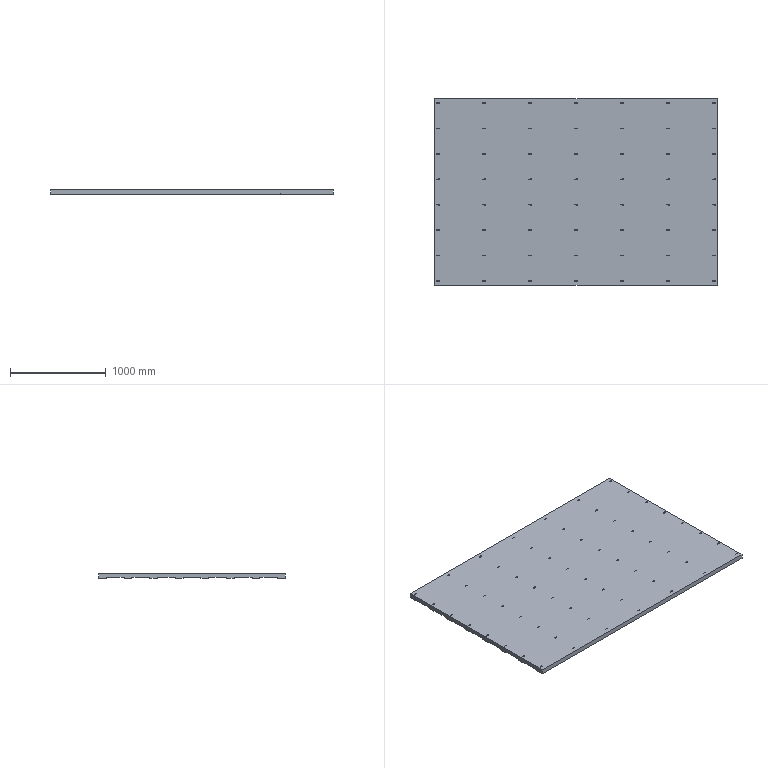Part | SolidWorks | features LPattern 4, ICE 2, FlatPattern 1, HoleWzd 1, SMBaseFlange 1, SheetMetal 1 | 1 solid | 674 faces | box 2950 x 1950 x 50 mm | volume 248660508 mm3 | cylinder 432 | cone 208 | plane 34 | commonest cylinder face diameters 6.8 x208 4 x112 10 x112